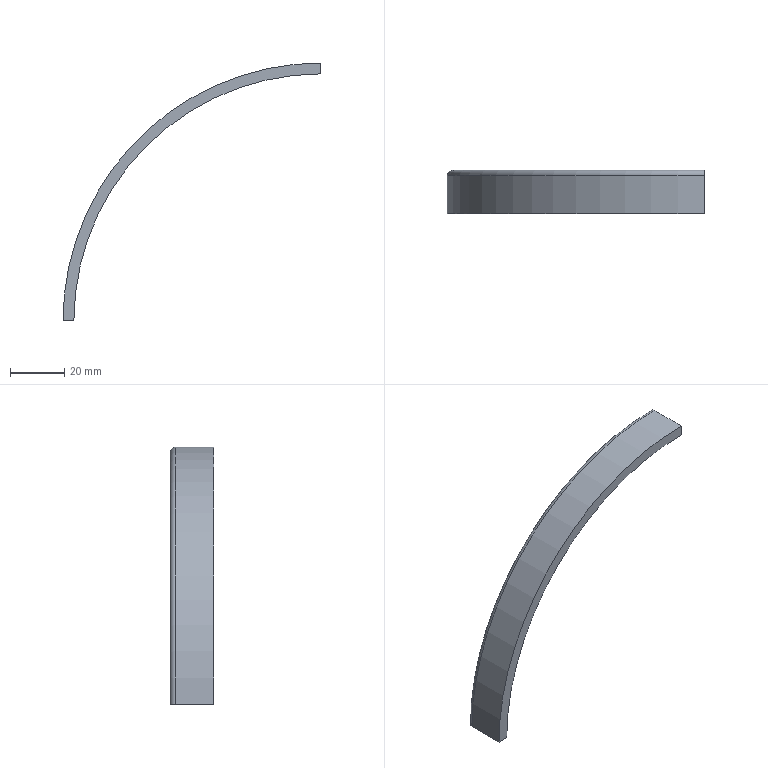Part | SolidWorks | features MirrorStock 1 | 1 solid | 7 faces | box 95 x 16 x 95 mm | volume 9099 mm3 | plane 3 | cylinder 2 | torus 2 | commonest cylinder face diameters 182 x1 190 x1
STEP:
#1=CARTESIAN_POINT('',(-95.,6.,0.));
#2=VERTEX_POINT('',#1);
#3=CARTESIAN_POINT('',(-95.,-8.,0.));
#4=VERTEX_POINT('',#3);
#5=CARTESIAN_POINT('',(-95.,8.,0.));
#6=DIRECTION('',(0.,-1.,0.));
#7=VECTOR('',#6,1000.);
#8=LINE('',#5,#7);
#9=EDGE_CURVE('',#2,#4,#8,.T.);
#10=ORIENTED_EDGE('',*,*,#9,.T.);
#11=CARTESIAN_POINT('',(0.,-8.,95.));
#12=VERTEX_POINT('',#11);
#13=CARTESIAN_POINT('',(0.,-8.,0.));
#14=DIRECTION('',(0.,-1.,0.));
#15=DIRECTION('',(0.,0.,-1.));
#16=AXIS2_PLACEMENT_3D('',#13,#14,#15);
#17=CIRCLE('',#16,95.);
#18=EDGE_CURVE('',#12,#4,#17,.T.);
#19=ORIENTED_EDGE('',*,*,#18,.F.);
#20=CARTESIAN_POINT('',(0.,6.,95.));
#21=VERTEX_POINT('',#20);
#22=CARTESIAN_POINT('',(0.,8.,95.));
#23=DIRECTION('',(0.,-1.,0.));
#24=VECTOR('',#23,1000.);
#25=LINE('',#22,#24);
#26=EDGE_CURVE('',#21,#12,#25,.T.);
#27=ORIENTED_EDGE('',*,*,#26,.F.);
#28=CARTESIAN_POINT('',(0.,6.,0.));
#29=DIRECTION('',(0.,1.,0.));
#30=DIRECTION('',(0.,0.,-1.));
#31=AXIS2_PLACEMENT_3D('',#28,#29,#30);
#32=CIRCLE('',#31,95.);
#33=EDGE_CURVE('',#2,#21,#32,.T.);
#34=ORIENTED_EDGE('',*,*,#33,.F.);
#35=EDGE_LOOP('',(#10,#19,#27,#34));
#36=FACE_OUTER_BOUND('',#35,.T.);
#37=CARTESIAN_POINT('',(0.,8.,0.));
#38=DIRECTION('',(0.,-1.,0.));
#39=DIRECTION('',(0.,0.,1.));
#40=AXIS2_PLACEMENT_3D('',#37,#38,#39);
#41=CYLINDRICAL_SURFACE('',#40,95.);
#42=ADVANCED_FACE('',(#36),#41,.T.);
#43=CARTESIAN_POINT('',(-91.,6.,0.));
#44=VERTEX_POINT('',#43);
#45=CARTESIAN_POINT('',(-93.,8.,0.));
#46=VERTEX_POINT('',#45);
#47=CARTESIAN_POINT('',(-93.,6.,0.));
#48=DIRECTION('',(0.,0.,1.));
#49=DIRECTION('',(-1.,0.,0.));
#50=AXIS2_PLACEMENT_3D('',#47,#48,#49);
#51=CIRCLE('',#50,2.);
#52=EDGE_CURVE('',#44,#46,#51,.T.);
#53=ORIENTED_EDGE('',*,*,#52,.F.);
#54=CARTESIAN_POINT('',(-91.,-8.,0.));
#55=VERTEX_POINT('',#54);
#56=CARTESIAN_POINT('',(-91.,8.,0.));
#57=DIRECTION('',(0.,-1.,0.));
#58=VECTOR('',#57,1000.);
#59=LINE('',#56,#58);
#60=EDGE_CURVE('',#44,#55,#59,.T.);
#61=ORIENTED_EDGE('',*,*,#60,.T.);
#62=CARTESIAN_POINT('',(-95.,-8.,0.));
#63=DIRECTION('',(1.,0.,0.));
#64=VECTOR('',#63,1000.);
#65=LINE('',#62,#64);
#66=EDGE_CURVE('',#4,#55,#65,.T.);
#67=ORIENTED_EDGE('',*,*,#66,.F.);
#68=ORIENTED_EDGE('',*,*,#9,.F.);
#69=CARTESIAN_POINT('',(-93.,6.,0.));
#70=DIRECTION('',(0.,0.,1.));
#71=DIRECTION('',(-1.,0.,0.));
#72=AXIS2_PLACEMENT_3D('',#69,#70,#71);
#73=CIRCLE('',#72,2.);
#74=EDGE_CURVE('',#46,#2,#73,.T.);
#75=ORIENTED_EDGE('',*,*,#74,.F.);
#76=EDGE_LOOP('',(#53,#61,#67,#68,#75));
#77=FACE_OUTER_BOUND('',#76,.T.);
#78=CARTESIAN_POINT('',(-95.,8.,0.));
#79=DIRECTION('',(0.,0.,1.));
#80=DIRECTION('',(-1.,0.,0.));
#81=AXIS2_PLACEMENT_3D('',#78,#79,#80);
#82=PLANE('',#81);
#83=ADVANCED_FACE('',(#77),#82,.F.);
#84=CARTESIAN_POINT('',(0.,6.,91.));
#85=VERTEX_POINT('',#84);
#86=CARTESIAN_POINT('',(0.,-8.,91.));
#87=VERTEX_POINT('',#86);
#88=CARTESIAN_POINT('',(0.,8.,91.));
#89=DIRECTION('',(0.,-1.,0.));
#90=VECTOR('',#89,1000.);
#91=LINE('',#88,#90);
#92=EDGE_CURVE('',#85,#87,#91,.T.);
#93=ORIENTED_EDGE('',*,*,#92,.T.);
#94=CARTESIAN_POINT('',(0.,-8.,0.));
#95=DIRECTION('',(0.,1.,0.));
#96=DIRECTION('',(0.,0.,-1.));
#97=AXIS2_PLACEMENT_3D('',#94,#95,#96);
#98=CIRCLE('',#97,91.);
#99=EDGE_CURVE('',#55,#87,#98,.T.);
#100=ORIENTED_EDGE('',*,*,#99,.F.);
#101=ORIENTED_EDGE('',*,*,#60,.F.);
#102=CARTESIAN_POINT('',(0.,6.,0.));
#103=DIRECTION('',(0.,-1.,0.));
#104=DIRECTION('',(0.,0.,-1.));
#105=AXIS2_PLACEMENT_3D('',#102,#103,#104);
#106=CIRCLE('',#105,91.);
#107=EDGE_CURVE('',#85,#44,#106,.T.);
#108=ORIENTED_EDGE('',*,*,#107,.F.);
#109=EDGE_LOOP('',(#93,#100,#101,#108));
#110=FACE_OUTER_BOUND('',#109,.T.);
#111=CARTESIAN_POINT('',(0.,8.,0.));
#112=DIRECTION('',(0.,-1.,0.));
#113=DIRECTION('',(0.,0.,1.));
#114=AXIS2_PLACEMENT_3D('',#111,#112,#113);
#115=CYLINDRICAL_SURFACE('',#114,91.);
#116=ADVANCED_FACE('',(#110),#115,.F.);
#117=ORIENTED_EDGE('',*,*,#26,.T.);
#118=CARTESIAN_POINT('',(0.,-8.,95.));
#119=DIRECTION('',(0.,0.,1.));
#120=VECTOR('',#119,1000.);
#121=LINE('',#118,#120);
#122=EDGE_CURVE('',#87,#12,#121,.T.);
#123=ORIENTED_EDGE('',*,*,#122,.F.);
#124=ORIENTED_EDGE('',*,*,#92,.F.);
#125=CARTESIAN_POINT('',(0.,8.,93.));
#126=VERTEX_POINT('',#125);
#127=CARTESIAN_POINT('',(0.,6.,93.));
#128=DIRECTION('',(-1.,0.,0.));
#129=DIRECTION('',(0.,0.,-1.));
#130=AXIS2_PLACEMENT_3D('',#127,#128,#129);
#131=CIRCLE('',#130,2.);
#132=EDGE_CURVE('',#126,#85,#131,.T.);
#133=ORIENTED_EDGE('',*,*,#132,.F.);
#134=CARTESIAN_POINT('',(0.,6.,93.));
#135=DIRECTION('',(-1.,0.,0.));
#136=DIRECTION('',(0.,0.,-1.));
#137=AXIS2_PLACEMENT_3D('',#134,#135,#136);
#138=CIRCLE('',#137,2.);
#139=EDGE_CURVE('',#21,#126,#138,.T.);
#140=ORIENTED_EDGE('',*,*,#139,.F.);
#141=EDGE_LOOP('',(#117,#123,#124,#133,#140));
#142=FACE_OUTER_BOUND('',#141,.T.);
#143=CARTESIAN_POINT('',(0.,8.,95.));
#144=DIRECTION('',(-1.,0.,0.));
#145=DIRECTION('',(0.,0.,-1.));
#146=AXIS2_PLACEMENT_3D('',#143,#144,#145);
#147=PLANE('',#146);
#148=ADVANCED_FACE('',(#142),#147,.F.);
#149=ORIENTED_EDGE('',*,*,#18,.T.);
#150=ORIENTED_EDGE('',*,*,#66,.T.);
#151=ORIENTED_EDGE('',*,*,#99,.T.);
#152=ORIENTED_EDGE('',*,*,#122,.T.);
#153=EDGE_LOOP('',(#149,#150,#151,#152));
#154=FACE_OUTER_BOUND('',#153,.T.);
#155=CARTESIAN_POINT('',(0.,-8.,0.));
#156=DIRECTION('',(0.,1.,0.));
#157=DIRECTION('',(0.,0.,-1.));
#158=AXIS2_PLACEMENT_3D('',#155,#156,#157);
#159=PLANE('',#158);
#160=ADVANCED_FACE('',(#154),#159,.F.);
#161=ORIENTED_EDGE('',*,*,#107,.T.);
#162=ORIENTED_EDGE('',*,*,#52,.T.);
#163=CARTESIAN_POINT('',(0.,8.,0.));
#164=DIRECTION('',(0.,1.,0.));
#165=DIRECTION('',(0.,0.,-1.));
#166=AXIS2_PLACEMENT_3D('',#163,#164,#165);
#167=CIRCLE('',#166,93.);
#168=EDGE_CURVE('',#46,#126,#167,.T.);
#169=ORIENTED_EDGE('',*,*,#168,.T.);
#170=ORIENTED_EDGE('',*,*,#132,.T.);
#171=EDGE_LOOP('',(#161,#162,#169,#170));
#172=FACE_OUTER_BOUND('',#171,.T.);
#173=CARTESIAN_POINT('',(0.,6.,0.));
#174=DIRECTION('',(0.,1.,0.));
#175=DIRECTION('',(0.,0.,-1.));
#176=AXIS2_PLACEMENT_3D('',#173,#174,#175);
#177=TOROIDAL_SURFACE('',#176,93.,2.);
#178=ADVANCED_FACE('',(#172),#177,.T.);
#179=ORIENTED_EDGE('',*,*,#139,.T.);
#180=ORIENTED_EDGE('',*,*,#168,.F.);
#181=ORIENTED_EDGE('',*,*,#74,.T.);
#182=ORIENTED_EDGE('',*,*,#33,.T.);
#183=EDGE_LOOP('',(#179,#180,#181,#182));
#184=FACE_OUTER_BOUND('',#183,.T.);
#185=CARTESIAN_POINT('',(0.,6.,0.));
#186=DIRECTION('',(0.,1.,0.));
#187=DIRECTION('',(0.,0.,-1.));
#188=AXIS2_PLACEMENT_3D('',#185,#186,#187);
#189=TOROIDAL_SURFACE('',#188,93.,2.);
#190=ADVANCED_FACE('',(#184),#189,.T.);
#191=CLOSED_SHELL('',(#42,#83,#116,#148,#160,#178,#190));
#192=MANIFOLD_SOLID_BREP('',#191);
#193=CARTESIAN_POINT('',(0.,0.,0.));
#194=DIRECTION('',(0.,0.,1.));
#195=DIRECTION('',(1.,0.,0.));
#196=AXIS2_PLACEMENT_3D('',#193,#194,#195);
#197=(LENGTH_UNIT()NAMED_UNIT(*)SI_UNIT(.MILLI.,.METRE.));
#198=UNCERTAINTY_MEASURE_WITH_UNIT(LENGTH_MEASURE(0.00001),#197,'','');
#199=(NAMED_UNIT(*)PLANE_ANGLE_UNIT()SI_UNIT($,.RADIAN.));
#200=(NAMED_UNIT(*)SI_UNIT($,.STERADIAN.)SOLID_ANGLE_UNIT());
#201=(GEOMETRIC_REPRESENTATION_CONTEXT(3)GLOBAL_UNCERTAINTY_ASSIGNED_CONTEXT((#198))GLOBAL_UNIT_ASSIGNED_CONTEXT((#197,#199,#200))REPRESENTATION_CONTEXT('',''));
#202=ADVANCED_BREP_SHAPE_REPRESENTATION('',(#192,#196),#201);